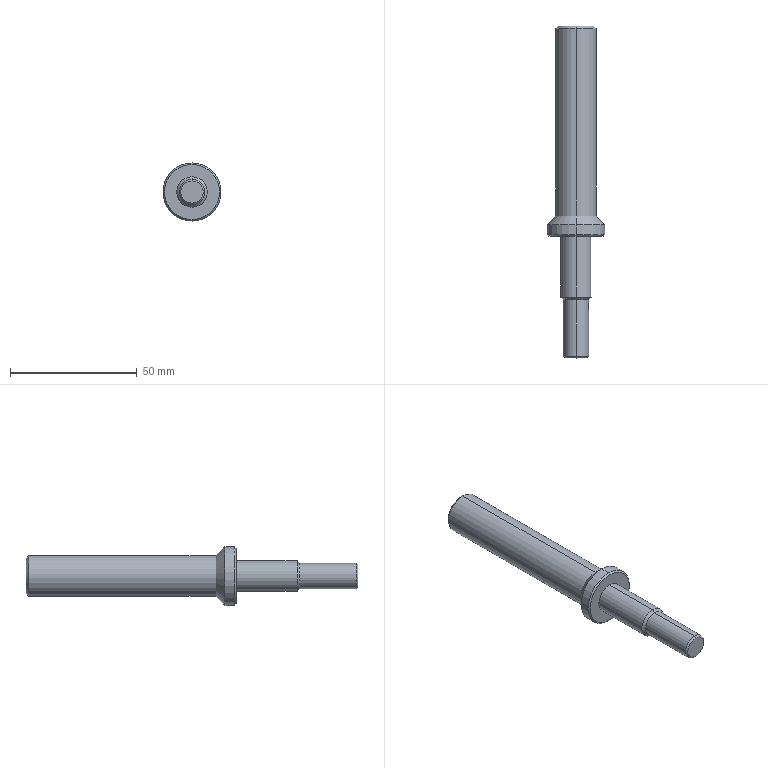Part | SolidWorks | features BaseBody 1 | 1 solid | 23 faces | box 23 x 131 x 23 mm | volume 22576 mm3 | cone 12 | cylinder 8 | plane 3 | commonest cylinder face diameters 10 x2 12 x2 16 x2 23 x2
STEP:
#1=CARTESIAN_POINT('',(0.,56.,8.));
#2=VERTEX_POINT('',#1);
#3=CARTESIAN_POINT('',(0.,56.,-8.));
#4=VERTEX_POINT('',#3);
#5=CARTESIAN_POINT('',(0.,56.,0.));
#6=DIRECTION('',(0.,1.,0.));
#7=DIRECTION('',(0.,0.,1.));
#8=AXIS2_PLACEMENT_3D('',#5,#6,#7);
#9=CIRCLE('',#8,8.);
#10=EDGE_CURVE('',#2,#4,#9,.T.);
#11=ORIENTED_EDGE('',*,*,#10,.T.);
#12=CARTESIAN_POINT('',(0.,130.,-8.));
#13=VERTEX_POINT('',#12);
#14=CARTESIAN_POINT('',(0.,131.,-8.));
#15=DIRECTION('',(0.,1.,0.));
#16=VECTOR('',#15,1000.);
#17=LINE('',#14,#16);
#18=EDGE_CURVE('',#4,#13,#17,.T.);
#19=ORIENTED_EDGE('',*,*,#18,.T.);
#20=CARTESIAN_POINT('',(0.,130.,8.));
#21=VERTEX_POINT('',#20);
#22=CARTESIAN_POINT('',(0.,130.,0.));
#23=DIRECTION('',(0.,-1.,0.));
#24=DIRECTION('',(0.,0.,1.));
#25=AXIS2_PLACEMENT_3D('',#22,#23,#24);
#26=CIRCLE('',#25,8.);
#27=EDGE_CURVE('',#13,#21,#26,.T.);
#28=ORIENTED_EDGE('',*,*,#27,.T.);
#29=CARTESIAN_POINT('',(0.,131.,8.));
#30=DIRECTION('',(0.,1.,0.));
#31=VECTOR('',#30,1000.);
#32=LINE('',#29,#31);
#33=EDGE_CURVE('',#2,#21,#32,.T.);
#34=ORIENTED_EDGE('',*,*,#33,.F.);
#35=EDGE_LOOP('',(#11,#19,#28,#34));
#36=FACE_OUTER_BOUND('',#35,.T.);
#37=CARTESIAN_POINT('',(0.,131.,0.));
#38=DIRECTION('',(0.,1.,0.));
#39=DIRECTION('',(0.,0.,1.));
#40=AXIS2_PLACEMENT_3D('',#37,#38,#39);
#41=CYLINDRICAL_SURFACE('',#40,8.);
#42=ADVANCED_FACE('',(#36),#41,.T.);
#43=CARTESIAN_POINT('',(0.,131.,-7.));
#44=VERTEX_POINT('',#43);
#45=CARTESIAN_POINT('',(0.,131.,7.));
#46=VERTEX_POINT('',#45);
#47=CARTESIAN_POINT('',(0.,131.,0.));
#48=DIRECTION('',(0.,-1.,0.));
#49=DIRECTION('',(0.,0.,-1.));
#50=AXIS2_PLACEMENT_3D('',#47,#48,#49);
#51=CIRCLE('',#50,7.);
#52=EDGE_CURVE('',#44,#46,#51,.T.);
#53=ORIENTED_EDGE('',*,*,#52,.T.);
#54=CARTESIAN_POINT('',(0.,130.,8.));
#55=DIRECTION('',(0.,-0.7071,0.7071));
#56=VECTOR('',#55,1000.);
#57=LINE('',#54,#56);
#58=EDGE_CURVE('',#46,#21,#57,.T.);
#59=ORIENTED_EDGE('',*,*,#58,.T.);
#60=ORIENTED_EDGE('',*,*,#27,.F.);
#61=CARTESIAN_POINT('',(0.,130.,-8.));
#62=DIRECTION('',(0.,-0.7071,-0.7071));
#63=VECTOR('',#62,1000.);
#64=LINE('',#61,#63);
#65=EDGE_CURVE('',#44,#13,#64,.T.);
#66=ORIENTED_EDGE('',*,*,#65,.F.);
#67=EDGE_LOOP('',(#53,#59,#60,#66));
#68=FACE_OUTER_BOUND('',#67,.T.);
#69=CARTESIAN_POINT('',(0.,130.,0.));
#70=DIRECTION('',(0.,-1.,0.));
#71=DIRECTION('',(0.,0.,-1.));
#72=AXIS2_PLACEMENT_3D('',#69,#70,#71);
#73=CONICAL_SURFACE('',#72,8.,0.7854);
#74=ADVANCED_FACE('',(#68),#73,.T.);
#75=ORIENTED_EDGE('',*,*,#10,.F.);
#76=CARTESIAN_POINT('',(0.,52.5,11.5));
#77=VERTEX_POINT('',#76);
#78=CARTESIAN_POINT('',(0.,52.5,11.5));
#79=DIRECTION('',(0.,-0.7071,0.7071));
#80=VECTOR('',#79,1000.);
#81=LINE('',#78,#80);
#82=EDGE_CURVE('',#2,#77,#81,.T.);
#83=ORIENTED_EDGE('',*,*,#82,.T.);
#84=CARTESIAN_POINT('',(0.,52.5,-11.5));
#85=VERTEX_POINT('',#84);
#86=CARTESIAN_POINT('',(0.,52.5,0.));
#87=DIRECTION('',(0.,1.,0.));
#88=DIRECTION('',(1.,0.,0.));
#89=AXIS2_PLACEMENT_3D('',#86,#87,#88);
#90=CIRCLE('',#89,11.5);
#91=EDGE_CURVE('',#77,#85,#90,.T.);
#92=ORIENTED_EDGE('',*,*,#91,.T.);
#93=CARTESIAN_POINT('',(0.,52.5,-11.5));
#94=DIRECTION('',(0.,-0.7071,-0.7071));
#95=VECTOR('',#94,1000.);
#96=LINE('',#93,#95);
#97=EDGE_CURVE('',#4,#85,#96,.T.);
#98=ORIENTED_EDGE('',*,*,#97,.F.);
#99=EDGE_LOOP('',(#75,#83,#92,#98));
#100=FACE_OUTER_BOUND('',#99,.T.);
#101=CARTESIAN_POINT('',(0.,52.5,0.));
#102=DIRECTION('',(0.,-1.,0.));
#103=DIRECTION('',(0.,0.,-1.));
#104=AXIS2_PLACEMENT_3D('',#101,#102,#103);
#105=CONICAL_SURFACE('',#104,11.5,0.7854);
#106=ADVANCED_FACE('',(#100),#105,.T.);
#107=CARTESIAN_POINT('',(0.,48.6,11.5));
#108=VERTEX_POINT('',#107);
#109=CARTESIAN_POINT('',(0.,48.6,-11.5));
#110=VERTEX_POINT('',#109);
#111=CARTESIAN_POINT('',(0.,48.6,0.));
#112=DIRECTION('',(0.,1.,0.));
#113=DIRECTION('',(0.,0.,1.));
#114=AXIS2_PLACEMENT_3D('',#111,#112,#113);
#115=CIRCLE('',#114,11.5);
#116=EDGE_CURVE('',#108,#110,#115,.T.);
#117=ORIENTED_EDGE('',*,*,#116,.T.);
#118=CARTESIAN_POINT('',(0.,131.,-11.5));
#119=DIRECTION('',(0.,1.,0.));
#120=VECTOR('',#119,1000.);
#121=LINE('',#118,#120);
#122=EDGE_CURVE('',#110,#85,#121,.T.);
#123=ORIENTED_EDGE('',*,*,#122,.T.);
#124=ORIENTED_EDGE('',*,*,#91,.F.);
#125=CARTESIAN_POINT('',(0.,131.,11.5));
#126=DIRECTION('',(0.,1.,0.));
#127=VECTOR('',#126,1000.);
#128=LINE('',#125,#127);
#129=EDGE_CURVE('',#108,#77,#128,.T.);
#130=ORIENTED_EDGE('',*,*,#129,.F.);
#131=EDGE_LOOP('',(#117,#123,#124,#130));
#132=FACE_OUTER_BOUND('',#131,.T.);
#133=CARTESIAN_POINT('',(0.,131.,0.));
#134=DIRECTION('',(0.,1.,0.));
#135=DIRECTION('',(0.,0.,1.));
#136=AXIS2_PLACEMENT_3D('',#133,#134,#135);
#137=CYLINDRICAL_SURFACE('',#136,11.5);
#138=ADVANCED_FACE('',(#132),#137,.T.);
#139=CARTESIAN_POINT('',(0.,48.,10.9));
#140=VERTEX_POINT('',#139);
#141=CARTESIAN_POINT('',(0.,48.,-10.9));
#142=VERTEX_POINT('',#141);
#143=CARTESIAN_POINT('',(0.,48.,0.));
#144=DIRECTION('',(0.,1.,0.));
#145=DIRECTION('',(0.,0.,1.));
#146=AXIS2_PLACEMENT_3D('',#143,#144,#145);
#147=CIRCLE('',#146,10.9);
#148=EDGE_CURVE('',#140,#142,#147,.T.);
#149=ORIENTED_EDGE('',*,*,#148,.T.);
#150=CARTESIAN_POINT('',(0.,48.6,-11.5));
#151=DIRECTION('',(0.,0.7071,-0.7071));
#152=VECTOR('',#151,1000.);
#153=LINE('',#150,#152);
#154=EDGE_CURVE('',#142,#110,#153,.T.);
#155=ORIENTED_EDGE('',*,*,#154,.T.);
#156=ORIENTED_EDGE('',*,*,#116,.F.);
#157=CARTESIAN_POINT('',(0.,48.6,11.5));
#158=DIRECTION('',(0.,0.7071,0.7071));
#159=VECTOR('',#158,1000.);
#160=LINE('',#157,#159);
#161=EDGE_CURVE('',#140,#108,#160,.T.);
#162=ORIENTED_EDGE('',*,*,#161,.F.);
#163=EDGE_LOOP('',(#149,#155,#156,#162));
#164=FACE_OUTER_BOUND('',#163,.T.);
#165=CARTESIAN_POINT('',(0.,48.6,0.));
#166=DIRECTION('',(0.,1.,0.));
#167=DIRECTION('',(0.,0.,1.));
#168=AXIS2_PLACEMENT_3D('',#165,#166,#167);
#169=CONICAL_SURFACE('',#168,11.5,0.7854);
#170=ADVANCED_FACE('',(#164),#169,.T.);
#171=CARTESIAN_POINT('',(0.,24.,6.));
#172=VERTEX_POINT('',#171);
#173=CARTESIAN_POINT('',(0.,24.,-6.));
#174=VERTEX_POINT('',#173);
#175=CARTESIAN_POINT('',(0.,24.,0.));
#176=DIRECTION('',(0.,1.,0.));
#177=DIRECTION('',(0.,0.,1.));
#178=AXIS2_PLACEMENT_3D('',#175,#176,#177);
#179=CIRCLE('',#178,6.);
#180=EDGE_CURVE('',#172,#174,#179,.T.);
#181=ORIENTED_EDGE('',*,*,#180,.T.);
#182=CARTESIAN_POINT('',(0.,48.,-6.));
#183=VERTEX_POINT('',#182);
#184=CARTESIAN_POINT('',(0.,131.,-6.));
#185=DIRECTION('',(0.,1.,0.));
#186=VECTOR('',#185,1000.);
#187=LINE('',#184,#186);
#188=EDGE_CURVE('',#174,#183,#187,.T.);
#189=ORIENTED_EDGE('',*,*,#188,.T.);
#190=CARTESIAN_POINT('',(0.,48.,6.));
#191=VERTEX_POINT('',#190);
#192=CARTESIAN_POINT('',(0.,48.,0.));
#193=DIRECTION('',(0.,1.,0.));
#194=DIRECTION('',(0.,0.,1.));
#195=AXIS2_PLACEMENT_3D('',#192,#193,#194);
#196=CIRCLE('',#195,6.);
#197=EDGE_CURVE('',#191,#183,#196,.T.);
#198=ORIENTED_EDGE('',*,*,#197,.F.);
#199=CARTESIAN_POINT('',(0.,131.,6.));
#200=DIRECTION('',(0.,1.,0.));
#201=VECTOR('',#200,1000.);
#202=LINE('',#199,#201);
#203=EDGE_CURVE('',#172,#191,#202,.T.);
#204=ORIENTED_EDGE('',*,*,#203,.F.);
#205=EDGE_LOOP('',(#181,#189,#198,#204));
#206=FACE_OUTER_BOUND('',#205,.T.);
#207=CARTESIAN_POINT('',(0.,131.,0.));
#208=DIRECTION('',(0.,1.,0.));
#209=DIRECTION('',(0.,0.,1.));
#210=AXIS2_PLACEMENT_3D('',#207,#208,#209);
#211=CYLINDRICAL_SURFACE('',#210,6.);
#212=ADVANCED_FACE('',(#206),#211,.T.);
#213=CARTESIAN_POINT('',(0.,23.,5.));
#214=VERTEX_POINT('',#213);
#215=CARTESIAN_POINT('',(0.,23.,-5.));
#216=VERTEX_POINT('',#215);
#217=CARTESIAN_POINT('',(0.,23.,0.));
#218=DIRECTION('',(0.,1.,0.));
#219=DIRECTION('',(1.,0.,0.));
#220=AXIS2_PLACEMENT_3D('',#217,#218,#219);
#221=CIRCLE('',#220,5.);
#222=EDGE_CURVE('',#214,#216,#221,.T.);
#223=ORIENTED_EDGE('',*,*,#222,.T.);
#224=CARTESIAN_POINT('',(0.,24.,-6.));
#225=DIRECTION('',(0.,0.7071,-0.7071));
#226=VECTOR('',#225,1000.);
#227=LINE('',#224,#226);
#228=EDGE_CURVE('',#216,#174,#227,.T.);
#229=ORIENTED_EDGE('',*,*,#228,.T.);
#230=ORIENTED_EDGE('',*,*,#180,.F.);
#231=CARTESIAN_POINT('',(0.,24.,6.));
#232=DIRECTION('',(0.,0.7071,0.7071));
#233=VECTOR('',#232,1000.);
#234=LINE('',#231,#233);
#235=EDGE_CURVE('',#214,#172,#234,.T.);
#236=ORIENTED_EDGE('',*,*,#235,.F.);
#237=EDGE_LOOP('',(#223,#229,#230,#236));
#238=FACE_OUTER_BOUND('',#237,.T.);
#239=CARTESIAN_POINT('',(0.,24.,0.));
#240=DIRECTION('',(0.,1.,0.));
#241=DIRECTION('',(0.,0.,1.));
#242=AXIS2_PLACEMENT_3D('',#239,#240,#241);
#243=CONICAL_SURFACE('',#242,6.,0.7854);
#244=ADVANCED_FACE('',(#238),#243,.T.);
#245=CARTESIAN_POINT('',(4.822,20.5,-1.322));
#246=VERTEX_POINT('',#245);
#247=CARTESIAN_POINT('',(4.822,20.5,1.322));
#248=VERTEX_POINT('',#247);
#249=CARTESIAN_POINT('',(4.822,20.5,-1.322));
#250=CARTESIAN_POINT('',(4.822,20.313,-1.322));
#251=CARTESIAN_POINT('',(4.831,20.131,-1.292));
#252=CARTESIAN_POINT('',(4.862,19.779,-1.17));
#253=CARTESIAN_POINT('',(4.883,19.618,-1.082));
#254=CARTESIAN_POINT('',(4.929,19.333,-0.8455));
#255=CARTESIAN_POINT('',(4.953,19.215,-0.7033));
#256=CARTESIAN_POINT('',(4.98,19.089,-0.4554));
#257=CARTESIAN_POINT('',(4.987,19.057,-0.3695));
#258=CARTESIAN_POINT('',(4.997,19.012,-0.1907));
#259=CARTESIAN_POINT('',(5.,19.,-0.09695));
#260=CARTESIAN_POINT('',(5.,19.,0.09078));
#261=CARTESIAN_POINT('',(4.997,19.011,0.1824));
#262=CARTESIAN_POINT('',(4.988,19.054,0.3613));
#263=CARTESIAN_POINT('',(4.98,19.087,0.4497));
#264=CARTESIAN_POINT('',(4.954,19.211,0.6976));
#265=CARTESIAN_POINT('',(4.93,19.331,0.8433));
#266=CARTESIAN_POINT('',(4.884,19.614,1.079));
#267=CARTESIAN_POINT('',(4.862,19.778,1.169));
#268=CARTESIAN_POINT('',(4.831,20.128,1.291));
#269=CARTESIAN_POINT('',(4.822,20.313,1.322));
#270=CARTESIAN_POINT('',(4.822,20.5,1.322));
#271=B_SPLINE_CURVE_WITH_KNOTS('',3,(#249,#250,#251,#252,#253,#254,#255,#256,#257,#258,#259,#260,#261,#262,#263,#264,#265,#266,#267,#268,#269,#270),.UNSPECIFIED.,.F.,.F.,(4,2,2,2,2,2,2,2,2,2,4),(0.,0.0005528,0.001106,0.001658,0.001935,0.002211,0.002488,0.002764,0.003317,0.00387,0.004423),.UNSPECIFIED.);
#272=EDGE_CURVE('',#246,#248,#271,.T.);
#273=ORIENTED_EDGE('',*,*,#272,.T.);
#274=CARTESIAN_POINT('',(4.822,20.5,1.322));
#275=CARTESIAN_POINT('',(4.822,20.687,1.322));
#276=CARTESIAN_POINT('',(4.831,20.869,1.292));
#277=CARTESIAN_POINT('',(4.862,21.221,1.17));
#278=CARTESIAN_POINT('',(4.883,21.382,1.082));
#279=CARTESIAN_POINT('',(4.929,21.667,0.8455));
#280=CARTESIAN_POINT('',(4.953,21.785,0.7033));
#281=CARTESIAN_POINT('',(4.98,21.911,0.4554));
#282=CARTESIAN_POINT('',(4.987,21.943,0.3695));
#283=CARTESIAN_POINT('',(4.997,21.988,0.1907));
#284=CARTESIAN_POINT('',(5.,22.,0.09695));
#285=CARTESIAN_POINT('',(5.,22.,-0.09078));
#286=CARTESIAN_POINT('',(4.997,21.989,-0.1824));
#287=CARTESIAN_POINT('',(4.988,21.946,-0.3613));
#288=CARTESIAN_POINT('',(4.98,21.913,-0.4497));
#289=CARTESIAN_POINT('',(4.954,21.789,-0.6976));
#290=CARTESIAN_POINT('',(4.93,21.669,-0.8433));
#291=CARTESIAN_POINT('',(4.884,21.386,-1.079));
#292=CARTESIAN_POINT('',(4.862,21.222,-1.169));
#293=CARTESIAN_POINT('',(4.831,20.872,-1.291));
#294=CARTESIAN_POINT('',(4.822,20.687,-1.322));
#295=CARTESIAN_POINT('',(4.822,20.5,-1.322));
#296=B_SPLINE_CURVE_WITH_KNOTS('',3,(#274,#275,#276,#277,#278,#279,#280,#281,#282,#283,#284,#285,#286,#287,#288,#289,#290,#291,#292,#293,#294,#295),.UNSPECIFIED.,.F.,.F.,(4,2,2,2,2,2,2,2,2,2,4),(-0.004428,-0.003874,-0.003321,-0.002767,-0.002491,-0.002214,-0.001937,-0.00166,-0.001107,-0.0005535,0.),.UNSPECIFIED.);
#297=EDGE_CURVE('',#248,#246,#296,.T.);
#298=ORIENTED_EDGE('',*,*,#297,.T.);
#299=EDGE_LOOP('',(#273,#298));
#300=FACE_BOUND('',#299,.T.);
#301=CARTESIAN_POINT('',(0.,0.6,5.));
#302=VERTEX_POINT('',#301);
#303=CARTESIAN_POINT('',(0.,0.6,-5.));
#304=VERTEX_POINT('',#303);
#305=CARTESIAN_POINT('',(0.,0.6,0.));
#306=DIRECTION('',(0.,1.,0.));
#307=DIRECTION('',(0.,0.,1.));
#308=AXIS2_PLACEMENT_3D('',#305,#306,#307);
#309=CIRCLE('',#308,5.);
#310=EDGE_CURVE('',#302,#304,#309,.T.);
#311=ORIENTED_EDGE('',*,*,#310,.T.);
#312=CARTESIAN_POINT('',(0.,131.,-5.));
#313=DIRECTION('',(0.,1.,0.));
#314=VECTOR('',#313,1000.);
#315=LINE('',#312,#314);
#316=EDGE_CURVE('',#304,#216,#315,.T.);
#317=ORIENTED_EDGE('',*,*,#316,.T.);
#318=ORIENTED_EDGE('',*,*,#222,.F.);
#319=CARTESIAN_POINT('',(0.,131.,5.));
#320=DIRECTION('',(0.,1.,0.));
#321=VECTOR('',#320,1000.);
#322=LINE('',#319,#321);
#323=EDGE_CURVE('',#302,#214,#322,.T.);
#324=ORIENTED_EDGE('',*,*,#323,.F.);
#325=EDGE_LOOP('',(#311,#317,#318,#324));
#326=FACE_OUTER_BOUND('',#325,.T.);
#327=CARTESIAN_POINT('',(0.,131.,0.));
#328=DIRECTION('',(0.,1.,0.));
#329=DIRECTION('',(0.,0.,1.));
#330=AXIS2_PLACEMENT_3D('',#327,#328,#329);
#331=CYLINDRICAL_SURFACE('',#330,5.);
#332=ADVANCED_FACE('',(#300,#326),#331,.T.);
#333=CARTESIAN_POINT('',(3.5,20.5,0.));
#334=VERTEX_POINT('',#333);
#335=CARTESIAN_POINT('',(5.009,20.5,-1.509));
#336=DIRECTION('',(0.7071,0.,-0.7071));
#337=VECTOR('',#336,1000.);
#338=LINE('',#335,#337);
#339=EDGE_CURVE('',#334,#246,#338,.T.);
#340=ORIENTED_EDGE('',*,*,#339,.F.);
#341=CARTESIAN_POINT('',(5.009,20.5,1.509));
#342=DIRECTION('',(0.7071,0.,0.7071));
#343=VECTOR('',#342,1000.);
#344=LINE('',#341,#343);
#345=EDGE_CURVE('',#334,#248,#344,.T.);
#346=ORIENTED_EDGE('',*,*,#345,.T.);
#347=ORIENTED_EDGE('',*,*,#272,.F.);
#348=EDGE_LOOP('',(#340,#346,#347));
#349=FACE_OUTER_BOUND('',#348,.T.);
#350=CARTESIAN_POINT('',(5.009,20.5,0.));
#351=DIRECTION('',(1.,0.,0.));
#352=DIRECTION('',(0.,0.,-1.));
#353=AXIS2_PLACEMENT_3D('',#350,#351,#352);
#354=CONICAL_SURFACE('',#353,1.509,0.7854);
#355=ADVANCED_FACE('',(#349),#354,.F.);
#356=CARTESIAN_POINT('',(0.,0.,4.4));
#357=VERTEX_POINT('',#356);
#358=CARTESIAN_POINT('',(0.,0.,-4.4));
#359=VERTEX_POINT('',#358);
#360=CARTESIAN_POINT('',(0.,0.,0.));
#361=DIRECTION('',(0.,1.,0.));
#362=DIRECTION('',(0.,0.,1.));
#363=AXIS2_PLACEMENT_3D('',#360,#361,#362);
#364=CIRCLE('',#363,4.4);
#365=EDGE_CURVE('',#357,#359,#364,.T.);
#366=ORIENTED_EDGE('',*,*,#365,.T.);
#367=CARTESIAN_POINT('',(0.,0.6,-5.));
#368=DIRECTION('',(0.,0.7071,-0.7071));
#369=VECTOR('',#368,1000.);
#370=LINE('',#367,#369);
#371=EDGE_CURVE('',#359,#304,#370,.T.);
#372=ORIENTED_EDGE('',*,*,#371,.T.);
#373=ORIENTED_EDGE('',*,*,#310,.F.);
#374=CARTESIAN_POINT('',(0.,0.6,5.));
#375=DIRECTION('',(0.,0.7071,0.7071));
#376=VECTOR('',#375,1000.);
#377=LINE('',#374,#376);
#378=EDGE_CURVE('',#357,#302,#377,.T.);
#379=ORIENTED_EDGE('',*,*,#378,.F.);
#380=EDGE_LOOP('',(#366,#372,#373,#379));
#381=FACE_OUTER_BOUND('',#380,.T.);
#382=CARTESIAN_POINT('',(0.,0.6,0.));
#383=DIRECTION('',(0.,1.,0.));
#384=DIRECTION('',(0.,0.,1.));
#385=AXIS2_PLACEMENT_3D('',#382,#383,#384);
#386=CONICAL_SURFACE('',#385,5.,0.7854);
#387=ADVANCED_FACE('',(#381),#386,.T.);
#388=ORIENTED_EDGE('',*,*,#18,.F.);
#389=CARTESIAN_POINT('',(0.,56.,0.));
#390=DIRECTION('',(0.,1.,0.));
#391=DIRECTION('',(0.,0.,1.));
#392=AXIS2_PLACEMENT_3D('',#389,#390,#391);
#393=CIRCLE('',#392,8.);
#394=EDGE_CURVE('',#4,#2,#393,.T.);
#395=ORIENTED_EDGE('',*,*,#394,.T.);
#396=ORIENTED_EDGE('',*,*,#33,.T.);
#397=CARTESIAN_POINT('',(0.,130.,0.));
#398=DIRECTION('',(0.,-1.,0.));
#399=DIRECTION('',(0.,0.,1.));
#400=AXIS2_PLACEMENT_3D('',#397,#398,#399);
#401=CIRCLE('',#400,8.);
#402=EDGE_CURVE('',#21,#13,#401,.T.);
#403=ORIENTED_EDGE('',*,*,#402,.T.);
#404=EDGE_LOOP('',(#388,#395,#396,#403));
#405=FACE_OUTER_BOUND('',#404,.T.);
#406=CARTESIAN_POINT('',(0.,131.,0.));
#407=DIRECTION('',(0.,1.,0.));
#408=DIRECTION('',(0.,0.,1.));
#409=AXIS2_PLACEMENT_3D('',#406,#407,#408);
#410=CYLINDRICAL_SURFACE('',#409,8.);
#411=ADVANCED_FACE('',(#405),#410,.T.);
#412=ORIENTED_EDGE('',*,*,#58,.F.);
#413=CARTESIAN_POINT('',(0.,131.,0.));
#414=DIRECTION('',(0.,-1.,0.));
#415=DIRECTION('',(0.,0.,-1.));
#416=AXIS2_PLACEMENT_3D('',#413,#414,#415);
#417=CIRCLE('',#416,7.);
#418=EDGE_CURVE('',#46,#44,#417,.T.);
#419=ORIENTED_EDGE('',*,*,#418,.T.);
#420=ORIENTED_EDGE('',*,*,#65,.T.);
#421=ORIENTED_EDGE('',*,*,#402,.F.);
#422=EDGE_LOOP('',(#412,#419,#420,#421));
#423=FACE_OUTER_BOUND('',#422,.T.);
#424=CARTESIAN_POINT('',(0.,130.,0.));
#425=DIRECTION('',(0.,-1.,0.));
#426=DIRECTION('',(0.,0.,-1.));
#427=AXIS2_PLACEMENT_3D('',#424,#425,#426);
#428=CONICAL_SURFACE('',#427,8.,0.7854);
#429=ADVANCED_FACE('',(#423),#428,.T.);
#430=ORIENTED_EDGE('',*,*,#82,.F.);
#431=ORIENTED_EDGE('',*,*,#394,.F.);
#432=ORIENTED_EDGE('',*,*,#97,.T.);
#433=CARTESIAN_POINT('',(0.,52.5,0.));
#434=DIRECTION('',(0.,1.,0.));
#435=DIRECTION('',(1.,0.,0.));
#436=AXIS2_PLACEMENT_3D('',#433,#434,#435);
#437=CIRCLE('',#436,11.5);
#438=EDGE_CURVE('',#85,#77,#437,.T.);
#439=ORIENTED_EDGE('',*,*,#438,.T.);
#440=EDGE_LOOP('',(#430,#431,#432,#439));
#441=FACE_OUTER_BOUND('',#440,.T.);
#442=CARTESIAN_POINT('',(0.,52.5,0.));
#443=DIRECTION('',(0.,-1.,0.));
#444=DIRECTION('',(0.,0.,-1.));
#445=AXIS2_PLACEMENT_3D('',#442,#443,#444);
#446=CONICAL_SURFACE('',#445,11.5,0.7854);
#447=ADVANCED_FACE('',(#441),#446,.T.);
#448=ORIENTED_EDGE('',*,*,#52,.F.);
#449=ORIENTED_EDGE('',*,*,#418,.F.);
#450=EDGE_LOOP('',(#448,#449));
#451=FACE_OUTER_BOUND('',#450,.T.);
#452=CARTESIAN_POINT('',(-7.,131.,0.));
#453=DIRECTION('',(0.,1.,0.));
#454=DIRECTION('',(-1.,0.,0.));
#455=AXIS2_PLACEMENT_3D('',#452,#453,#454);
#456=PLANE('',#455);
#457=ADVANCED_FACE('',(#451),#456,.T.);
#458=ORIENTED_EDGE('',*,*,#122,.F.);
#459=CARTESIAN_POINT('',(0.,48.6,0.));
#460=DIRECTION('',(0.,1.,0.));
#461=DIRECTION('',(0.,0.,1.));
#462=AXIS2_PLACEMENT_3D('',#459,#460,#461);
#463=CIRCLE('',#462,11.5);
#464=EDGE_CURVE('',#110,#108,#463,.T.);
#465=ORIENTED_EDGE('',*,*,#464,.T.);
#466=ORIENTED_EDGE('',*,*,#129,.T.);
#467=ORIENTED_EDGE('',*,*,#438,.F.);
#468=EDGE_LOOP('',(#458,#465,#466,#467));
#469=FACE_OUTER_BOUND('',#468,.T.);
#470=CARTESIAN_POINT('',(0.,131.,0.));
#471=DIRECTION('',(0.,1.,0.));
#472=DIRECTION('',(0.,0.,1.));
#473=AXIS2_PLACEMENT_3D('',#470,#471,#472);
#474=CYLINDRICAL_SURFACE('',#473,11.5);
#475=ADVANCED_FACE('',(#469),#474,.T.);
#476=ORIENTED_EDGE('',*,*,#154,.F.);
#477=CARTESIAN_POINT('',(0.,48.,0.));
#478=DIRECTION('',(0.,1.,0.));
#479=DIRECTION('',(0.,0.,1.));
#480=AXIS2_PLACEMENT_3D('',#477,#478,#479);
#481=CIRCLE('',#480,10.9);
#482=EDGE_CURVE('',#142,#140,#481,.T.);
#483=ORIENTED_EDGE('',*,*,#482,.T.);
#484=ORIENTED_EDGE('',*,*,#161,.T.);
#485=ORIENTED_EDGE('',*,*,#464,.F.);
#486=EDGE_LOOP('',(#476,#483,#484,#485));
#487=FACE_OUTER_BOUND('',#486,.T.);
#488=CARTESIAN_POINT('',(0.,48.6,0.));
#489=DIRECTION('',(0.,1.,0.));
#490=DIRECTION('',(0.,0.,1.));
#491=AXIS2_PLACEMENT_3D('',#488,#489,#490);
#492=CONICAL_SURFACE('',#491,11.5,0.7854);
#493=ADVANCED_FACE('',(#487),#492,.T.);
#494=ORIENTED_EDGE('',*,*,#197,.T.);
#495=CARTESIAN_POINT('',(0.,48.,0.));
#496=DIRECTION('',(0.,1.,0.));
#497=DIRECTION('',(0.,0.,1.));
#498=AXIS2_PLACEMENT_3D('',#495,#496,#497);
#499=CIRCLE('',#498,6.);
#500=EDGE_CURVE('',#183,#191,#499,.T.);
#501=ORIENTED_EDGE('',*,*,#500,.T.);
#502=EDGE_LOOP('',(#494,#501));
#503=FACE_BOUND('',#502,.T.);
#504=ORIENTED_EDGE('',*,*,#148,.F.);
#505=ORIENTED_EDGE('',*,*,#482,.F.);
#506=EDGE_LOOP('',(#504,#505));
#507=FACE_OUTER_BOUND('',#506,.T.);
#508=CARTESIAN_POINT('',(-6.,48.,0.));
#509=DIRECTION('',(0.,-1.,0.));
#510=DIRECTION('',(1.,0.,0.));
#511=AXIS2_PLACEMENT_3D('',#508,#509,#510);
#512=PLANE('',#511);
#513=ADVANCED_FACE('',(#503,#507),#512,.T.);
#514=ORIENTED_EDGE('',*,*,#188,.F.);
#515=CARTESIAN_POINT('',(0.,24.,0.));
#516=DIRECTION('',(0.,1.,0.));
#517=DIRECTION('',(0.,0.,1.));
#518=AXIS2_PLACEMENT_3D('',#515,#516,#517);
#519=CIRCLE('',#518,6.);
#520=EDGE_CURVE('',#174,#172,#519,.T.);
#521=ORIENTED_EDGE('',*,*,#520,.T.);
#522=ORIENTED_EDGE('',*,*,#203,.T.);
#523=ORIENTED_EDGE('',*,*,#500,.F.);
#524=EDGE_LOOP('',(#514,#521,#522,#523));
#525=FACE_OUTER_BOUND('',#524,.T.);
#526=CARTESIAN_POINT('',(0.,131.,0.));
#527=DIRECTION('',(0.,1.,0.));
#528=DIRECTION('',(0.,0.,1.));
#529=AXIS2_PLACEMENT_3D('',#526,#527,#528);
#530=CYLINDRICAL_SURFACE('',#529,6.);
#531=ADVANCED_FACE('',(#525),#530,.T.);
#532=ORIENTED_EDGE('',*,*,#228,.F.);
#533=CARTESIAN_POINT('',(0.,23.,0.));
#534=DIRECTION('',(0.,1.,0.));
#535=DIRECTION('',(1.,0.,0.));
#536=AXIS2_PLACEMENT_3D('',#533,#534,#535);
#537=CIRCLE('',#536,5.);
#538=EDGE_CURVE('',#216,#214,#537,.T.);
#539=ORIENTED_EDGE('',*,*,#538,.T.);
#540=ORIENTED_EDGE('',*,*,#235,.T.);
#541=ORIENTED_EDGE('',*,*,#520,.F.);
#542=EDGE_LOOP('',(#532,#539,#540,#541));
#543=FACE_OUTER_BOUND('',#542,.T.);
#544=CARTESIAN_POINT('',(0.,24.,0.));
#545=DIRECTION('',(0.,1.,0.));
#546=DIRECTION('',(0.,0.,1.));
#547=AXIS2_PLACEMENT_3D('',#544,#545,#546);
#548=CONICAL_SURFACE('',#547,6.,0.7854);
#549=ADVANCED_FACE('',(#543),#548,.T.);
#550=ORIENTED_EDGE('',*,*,#316,.F.);
#551=CARTESIAN_POINT('',(0.,0.6,0.));
#552=DIRECTION('',(0.,1.,0.));
#553=DIRECTION('',(0.,0.,1.));
#554=AXIS2_PLACEMENT_3D('',#551,#552,#553);
#555=CIRCLE('',#554,5.);
#556=EDGE_CURVE('',#304,#302,#555,.T.);
#557=ORIENTED_EDGE('',*,*,#556,.T.);
#558=ORIENTED_EDGE('',*,*,#323,.T.);
#559=ORIENTED_EDGE('',*,*,#538,.F.);
#560=EDGE_LOOP('',(#550,#557,#558,#559));
#561=FACE_OUTER_BOUND('',#560,.T.);
#562=CARTESIAN_POINT('',(0.,131.,0.));
#563=DIRECTION('',(0.,1.,0.));
#564=DIRECTION('',(0.,0.,1.));
#565=AXIS2_PLACEMENT_3D('',#562,#563,#564);
#566=CYLINDRICAL_SURFACE('',#565,5.);
#567=ADVANCED_FACE('',(#561),#566,.T.);
#568=ORIENTED_EDGE('',*,*,#345,.F.);
#569=ORIENTED_EDGE('',*,*,#339,.T.);
#570=ORIENTED_EDGE('',*,*,#297,.F.);
#571=EDGE_LOOP('',(#568,#569,#570));
#572=FACE_OUTER_BOUND('',#571,.T.);
#573=CARTESIAN_POINT('',(5.009,20.5,0.));
#574=DIRECTION('',(1.,0.,0.));
#575=DIRECTION('',(0.,0.,-1.));
#576=AXIS2_PLACEMENT_3D('',#573,#574,#575);
#577=CONICAL_SURFACE('',#576,1.509,0.7854);
#578=ADVANCED_FACE('',(#572),#577,.F.);
#579=ORIENTED_EDGE('',*,*,#371,.F.);
#580=CARTESIAN_POINT('',(0.,0.,0.));
#581=DIRECTION('',(0.,1.,0.));
#582=DIRECTION('',(0.,0.,1.));
#583=AXIS2_PLACEMENT_3D('',#580,#581,#582);
#584=CIRCLE('',#583,4.4);
#585=EDGE_CURVE('',#359,#357,#584,.T.);
#586=ORIENTED_EDGE('',*,*,#585,.T.);
#587=ORIENTED_EDGE('',*,*,#378,.T.);
#588=ORIENTED_EDGE('',*,*,#556,.F.);
#589=EDGE_LOOP('',(#579,#586,#587,#588));
#590=FACE_OUTER_BOUND('',#589,.T.);
#591=CARTESIAN_POINT('',(0.,0.6,0.));
#592=DIRECTION('',(0.,1.,0.));
#593=DIRECTION('',(0.,0.,1.));
#594=AXIS2_PLACEMENT_3D('',#591,#592,#593);
#595=CONICAL_SURFACE('',#594,5.,0.7854);
#596=ADVANCED_FACE('',(#590),#595,.T.);
#597=ORIENTED_EDGE('',*,*,#365,.F.);
#598=ORIENTED_EDGE('',*,*,#585,.F.);
#599=EDGE_LOOP('',(#597,#598));
#600=FACE_OUTER_BOUND('',#599,.T.);
#601=CARTESIAN_POINT('',(0.,0.,0.));
#602=DIRECTION('',(0.,-1.,0.));
#603=DIRECTION('',(1.,0.,0.));
#604=AXIS2_PLACEMENT_3D('',#601,#602,#603);
#605=PLANE('',#604);
#606=ADVANCED_FACE('',(#600),#605,.T.);
#607=CLOSED_SHELL('',(#42,#74,#106,#138,#170,#212,#244,#332,#355,#387,#411,#429,#447,#457,#475,#493,#513,#531,#549,#567,#578,#596,#606));
#608=MANIFOLD_SOLID_BREP('',#607);
#609=CARTESIAN_POINT('',(0.,0.,0.));
#610=DIRECTION('',(0.,0.,1.));
#611=DIRECTION('',(1.,0.,0.));
#612=AXIS2_PLACEMENT_3D('',#609,#610,#611);
#613=(LENGTH_UNIT()NAMED_UNIT(*)SI_UNIT(.MILLI.,.METRE.));
#614=UNCERTAINTY_MEASURE_WITH_UNIT(LENGTH_MEASURE(0.00001),#613,'','');
#615=(NAMED_UNIT(*)PLANE_ANGLE_UNIT()SI_UNIT($,.RADIAN.));
#616=(NAMED_UNIT(*)SI_UNIT($,.STERADIAN.)SOLID_ANGLE_UNIT());
#617=(GEOMETRIC_REPRESENTATION_CONTEXT(3)GLOBAL_UNCERTAINTY_ASSIGNED_CONTEXT((#614))GLOBAL_UNIT_ASSIGNED_CONTEXT((#613,#615,#616))REPRESENTATION_CONTEXT('',''));
#618=ADVANCED_BREP_SHAPE_REPRESENTATION('',(#608,#612),#617);